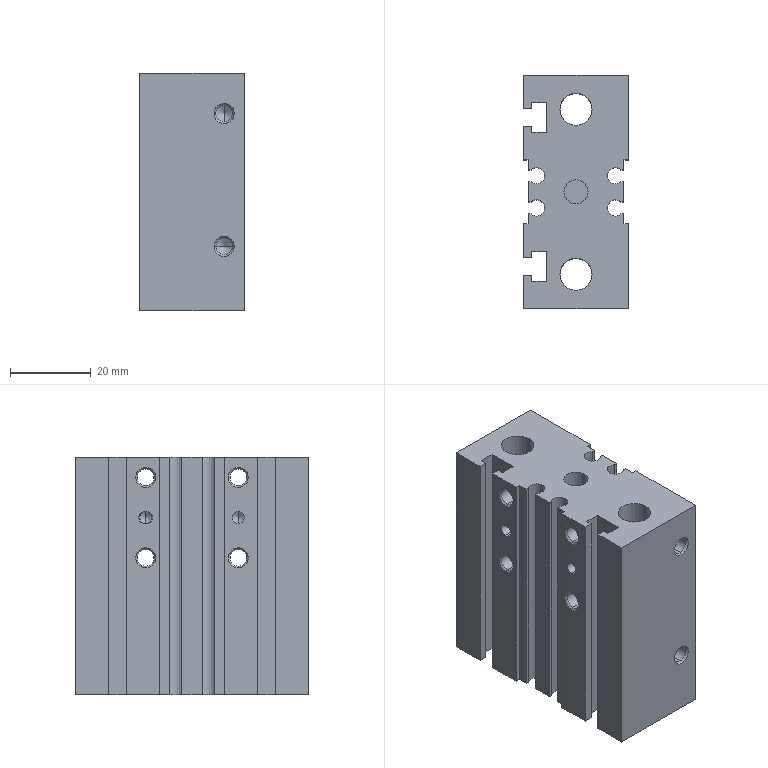Part | SolidWorks | features BaseBody 1 | 1 solid | 178 faces | box 26 x 58 x 59 mm | volume 66281 mm3 | cylinder 66 | plane 64 | cone 48 | commonest cylinder face diameters 4.134 x16 3 x12 8 x12 3.242 x8 4.3 x8 4.05 x6